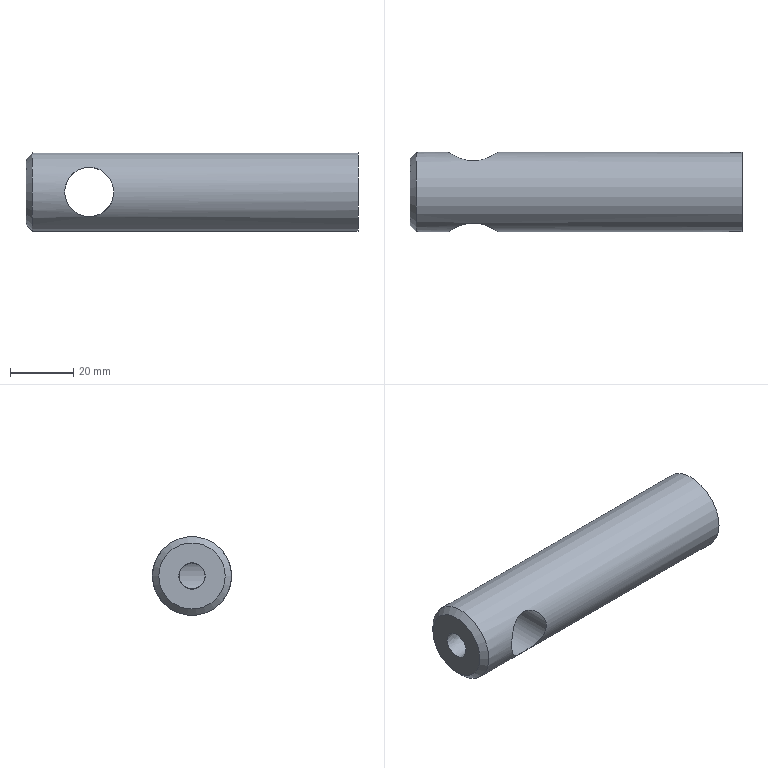Part | STEP file | support1 for guide-105 | 1 solid | 8 faces | box 105 x 25 x 25 mm | volume 45078 mm3 | spline 3 | cylinder 2 | plane 2 | cone 1 | commonest cylinder face diameters 15.5 x1 25 x1